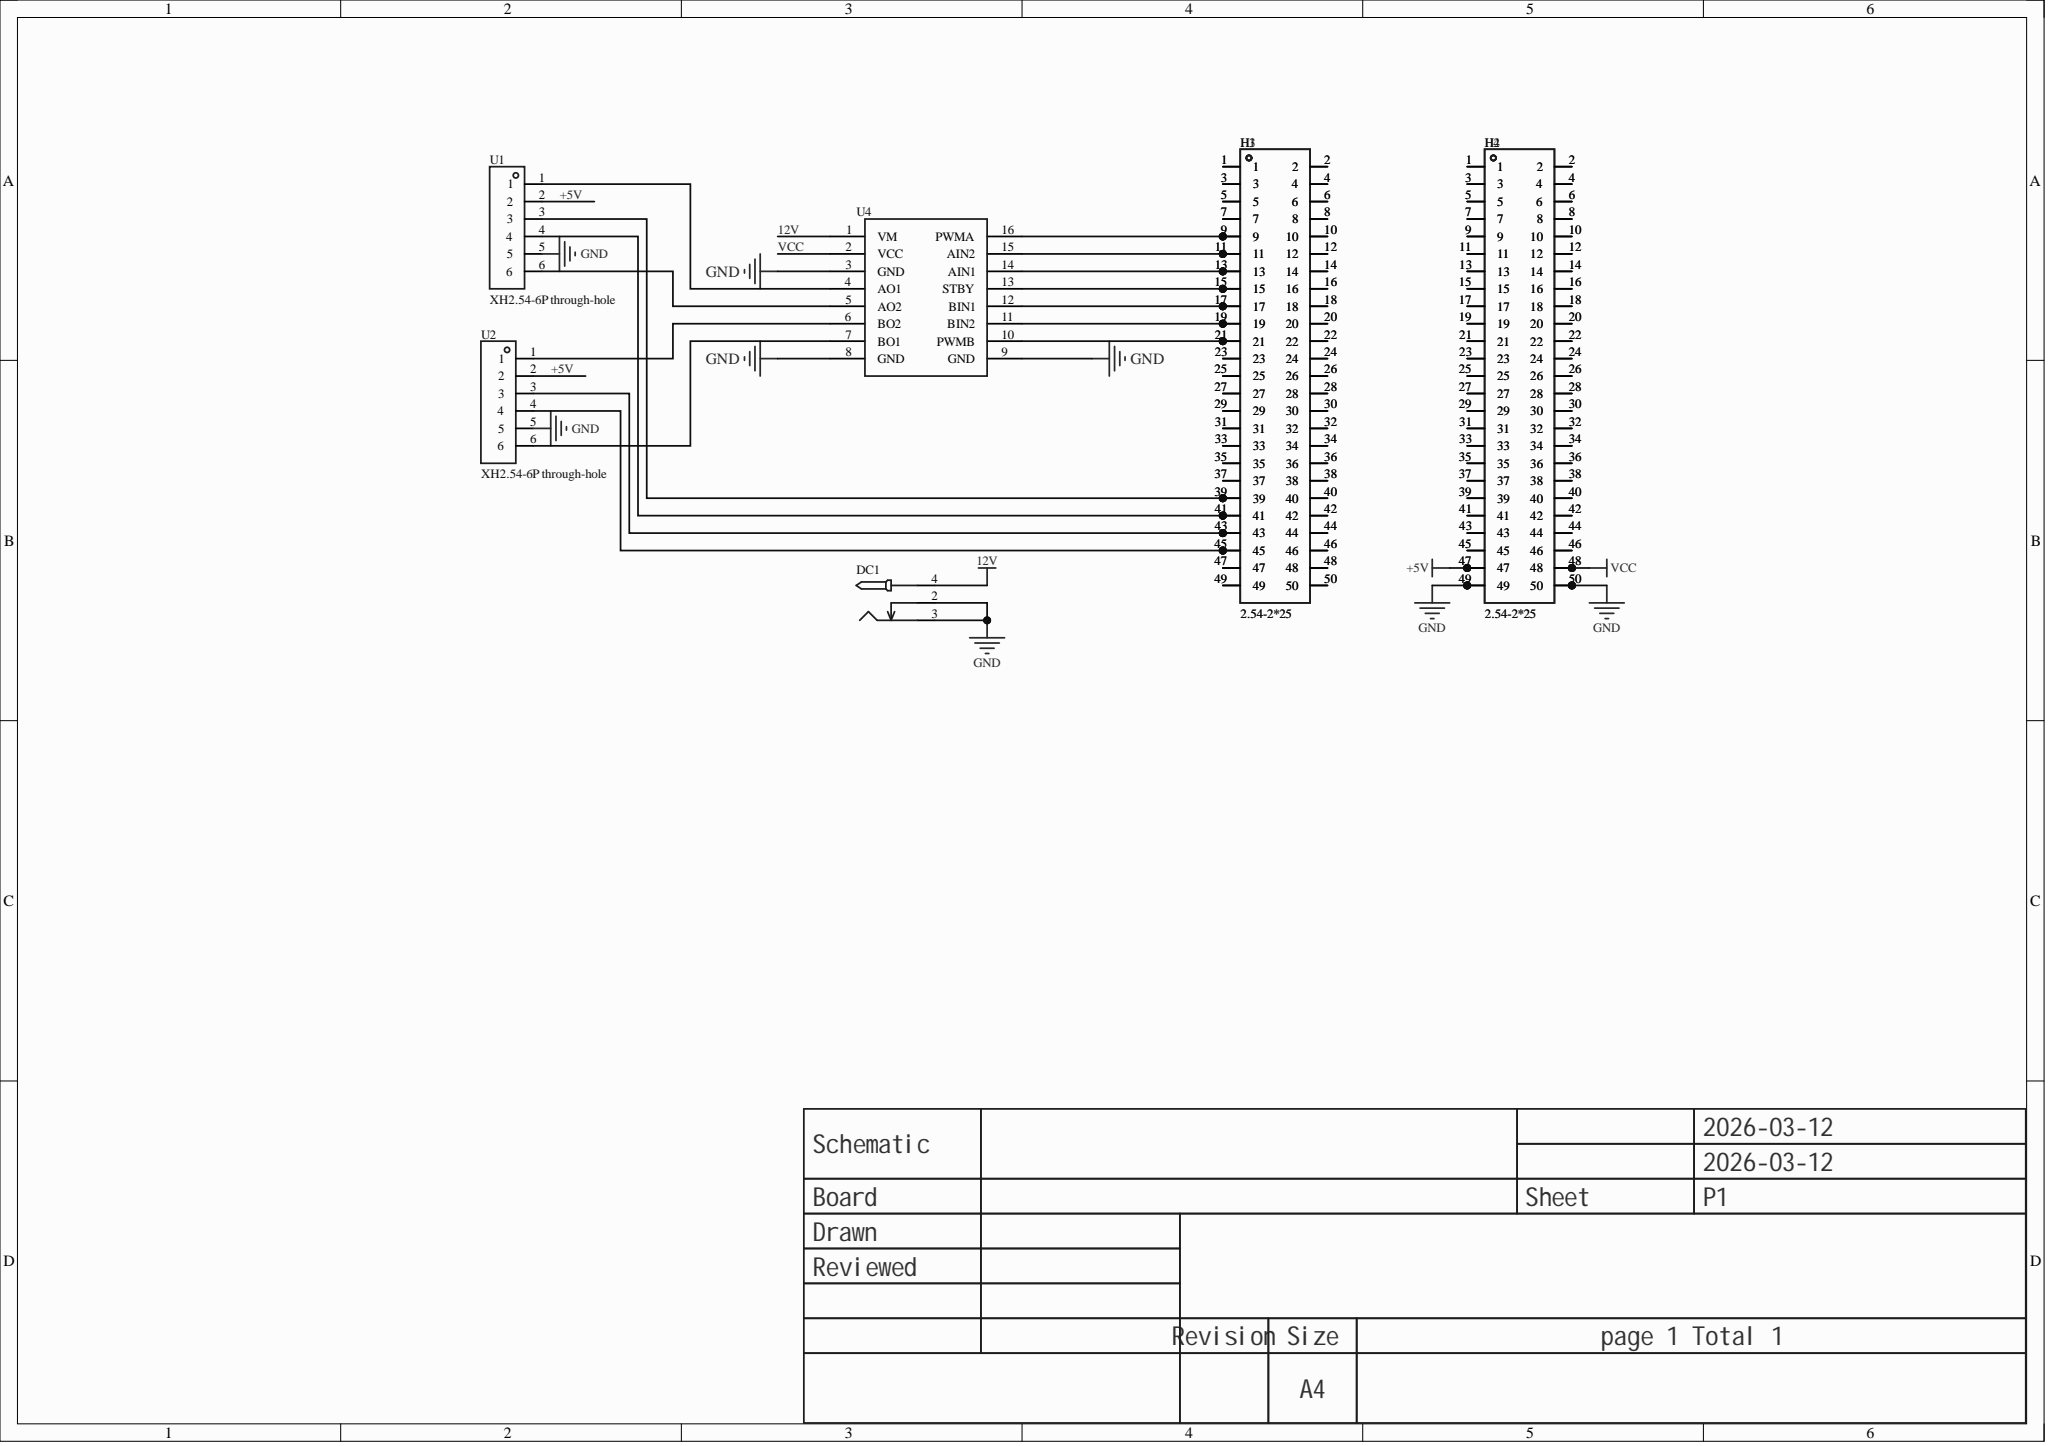Circuit board | Altium Designer | 8 parts | 104 nets
Bill of materials:
Comment,Description,Designator,Footprint,LibRef,Quantity
"","","DC1","DC-2.0","DC-005_2.0","1"
"2.54-2*25","插孔结构:2x25P;间距:2.54mm;行距:2.54mm;圆孔/方孔:方孔;安装方式:直插;排数:双排;总孔位数:50P;额定电流:2.5A;插孔方向:顶部;塑高:8.5mm;触头材质:黄铜;工作温度:-40℃~+105℃;","H1, H2, H3, H4","HDR-TH_50P-P2.54-V-F-R2-C25-S2.54-1","2.54-2*25","4"
"XH2.54-6P through-hole","","U1, U2","CONN-TH_XH2.54-6P","XH2.54-6P 直插","2"
"","","U4","tb6612","tb6612","1"
Netlist (Protel format):
[
DC1
DC-2.0




]
[
H1
HDR-TH_50P-P2.54-V-F-R2-C25-S2.54-1
2.54-2*25



]
[
H2
HDR-TH_50P-P2.54-V-F-R2-C25-S2.54-1
2.54-2*25



]
[
H3
HDR-TH_50P-P2.54-V-F-R2-C25-S2.54-1
2.54-2*25



]
[
H4
HDR-TH_50P-P2.54-V-F-R2-C25-S2.54-1
2.54-2*25



]
[
U1
CONN-TH_XH2.54-6P
XH2.54-6P through-hole



]
[
U2
CONN-TH_XH2.54-6P
XH2.54-6P through-hole



]
[
U4
tb6612




]
(
VCC
H2-48
H4-48
U4-2
)
(
NetU2_6
U2-6
U4-7
)
(
NetU2_1
U2-1
U4-6
)
(
NetU1_6
U1-6
U4-5
)
(
NetU1_1
U1-1
U4-4
)
(
NetH2_46
H2-46
H4-46
)
(
NetH2_45
H2-45
H4-45
)
(
NetH2_44
H2-44
H4-44
)
(
NetH2_43
H2-43
H4-43
)
(
NetH2_42
H2-42
H4-42
)
(
NetH2_41
H2-41
H4-41
)
(
NetH2_40
H2-40
H4-40
)
(
NetH2_39
H2-39
H4-39
)
(
NetH2_38
H2-38
H4-38
)
(
NetH2_37
H2-37
H4-37
)
(
NetH2_36
H2-36
H4-36
)
(
NetH2_35
H2-35
H4-35
)
(
NetH2_34
H2-34
H4-34
)
(
NetH2_33
H2-33
H4-33
)
(
NetH2_32
H2-32
H4-32
)
(
NetH2_31
H2-31
H4-31
)
(
NetH2_30
H2-30
H4-30
)
(
NetH2_29
H2-29
H4-29
)
(
NetH2_28
H2-28
H4-28
)
(
NetH2_27
H2-27
H4-27
)
(
NetH2_26
H2-26
H4-26
)
(
NetH2_25
H2-25
H4-25
)
(
NetH2_24
H2-24
H4-24
)
(
NetH2_23
H2-23
H4-23
)
(
NetH2_22
H2-22
H4-22
)
(
NetH2_21
H2-21
H4-21
)
(
NetH2_20
H2-20
H4-20
)
(
NetH2_19
H2-19
H4-19
)
(
NetH2_18
H2-18
H4-18
)
(
NetH2_17
H2-17
H4-17
)
(
NetH2_16
H2-16
H4-16
)
(
NetH2_15
H2-15
H4-15
)
(
NetH2_14
H2-14
H4-14
)
(
NetH2_13
H2-13
H4-13
)
(
NetH2_12
H2-12
H4-12
)
(
NetH2_11
H2-11
H4-11
)
(
NetH2_10
H2-10
H4-10
)
(
NetH2_9
H2-9
H4-9
)
(
NetH2_8
H2-8
H4-8
)
(
NetH2_7
H2-7
H4-7
)
(
NetH2_6
H2-6
H4-6
)
(
NetH2_5
H2-5
H4-5
)
(
NetH2_4
H2-4
H4-4
)
(
NetH2_3
H2-3
H4-3
)
(
NetH2_2
H2-2
H4-2
)
(
NetH2_1
H2-1
H4-1
)
(
NetH1_50
H1-50
H3-50
)
(
NetH1_49
H1-49
H3-49
)
(
NetH1_48
H1-48
H3-48
)
(
NetH1_47
H1-47
H3-47
)
(
NetH1_46
H1-46
H3-46
)
(
NetH1_45
H1-45
H3-45
U2-4
)
(
NetH1_44
H1-44
H3-44
)
(
NetH1_43
H1-43
H3-43
U2-3
)
(
NetH1_42
H1-42
H3-42
)
(
NetH1_41
H1-41
H3-41
U1-4
)
(
NetH1_40
H1-40
H3-40
)
(
NetH1_39
H1-39
H3-39
U1-3
)
(
NetH1_38
H1-38
H3-38
)
(
NetH1_37
H1-37
H3-37
)
(
NetH1_36
H1-36
H3-36
)
(
NetH1_35
H1-35
H3-35
)
(
NetH1_34
H1-34
H3-34
)
(
NetH1_33
H1-33
H3-33
)
(
NetH1_32
H1-32
H3-32
)
(
NetH1_31
H1-31
H3-31
)
(
NetH1_30
H1-30
H3-30
)
(
NetH1_29
H1-29
H3-29
)
(
NetH1_28
H1-28
H3-28
)
(
NetH1_27
H1-27
H3-27
)
(
NetH1_26
H1-26
H3-26
)
(
NetH1_25
H1-25
H3-25
)
(
NetH1_24
H1-24
H3-24
)
(
NetH1_23
H1-23
H3-23
)
(
NetH1_22
H1-22
H3-22
)
(
NetH1_21
H1-21
H3-21
U4-10
)
(
NetH1_20
H1-20
H3-20
)
(
NetH1_19
H1-19
H3-19
U4-11
)
(
NetH1_18
H1-18
H3-18
)
(
NetH1_17
H1-17
H3-17
U4-12
)
(
NetH1_16
H1-16
H3-16
)
(
NetH1_15
H1-15
H3-15
U4-13
)
(
NetH1_14
H1-14
H3-14
)
(
NetH1_13
H1-13
H3-13
U4-14
)
(
NetH1_12
H1-12
H3-12
)
(
NetH1_11
H1-11
H3-11
U4-15
)
(
NetH1_10
H1-10
H3-10
)
(
NetH1_9
H1-9
H3-9
U4-16
)
(
NetH1_8
H1-8
H3-8
)
(
NetH1_7
H1-7
H3-7
)
(
NetH1_6
H1-6
H3-6
)
(
NetH1_5
H1-5
H3-5
)
(
NetH1_4
H1-4
H3-4
)
(
NetH1_3
H1-3
H3-3
)
(
NetH1_2
H1-2
H3-2
)
(
NetH1_1
H1-1
H3-1
)
(
GND
DC1-2
DC1-3
H2-49
H2-50
H4-49
H4-50
U1-5
U2-5
U4-3
U4-8
U4-9
)
(
+5V
H2-47
H4-47
U1-2
U2-2
)
(
12V
DC1-4
U4-1
)